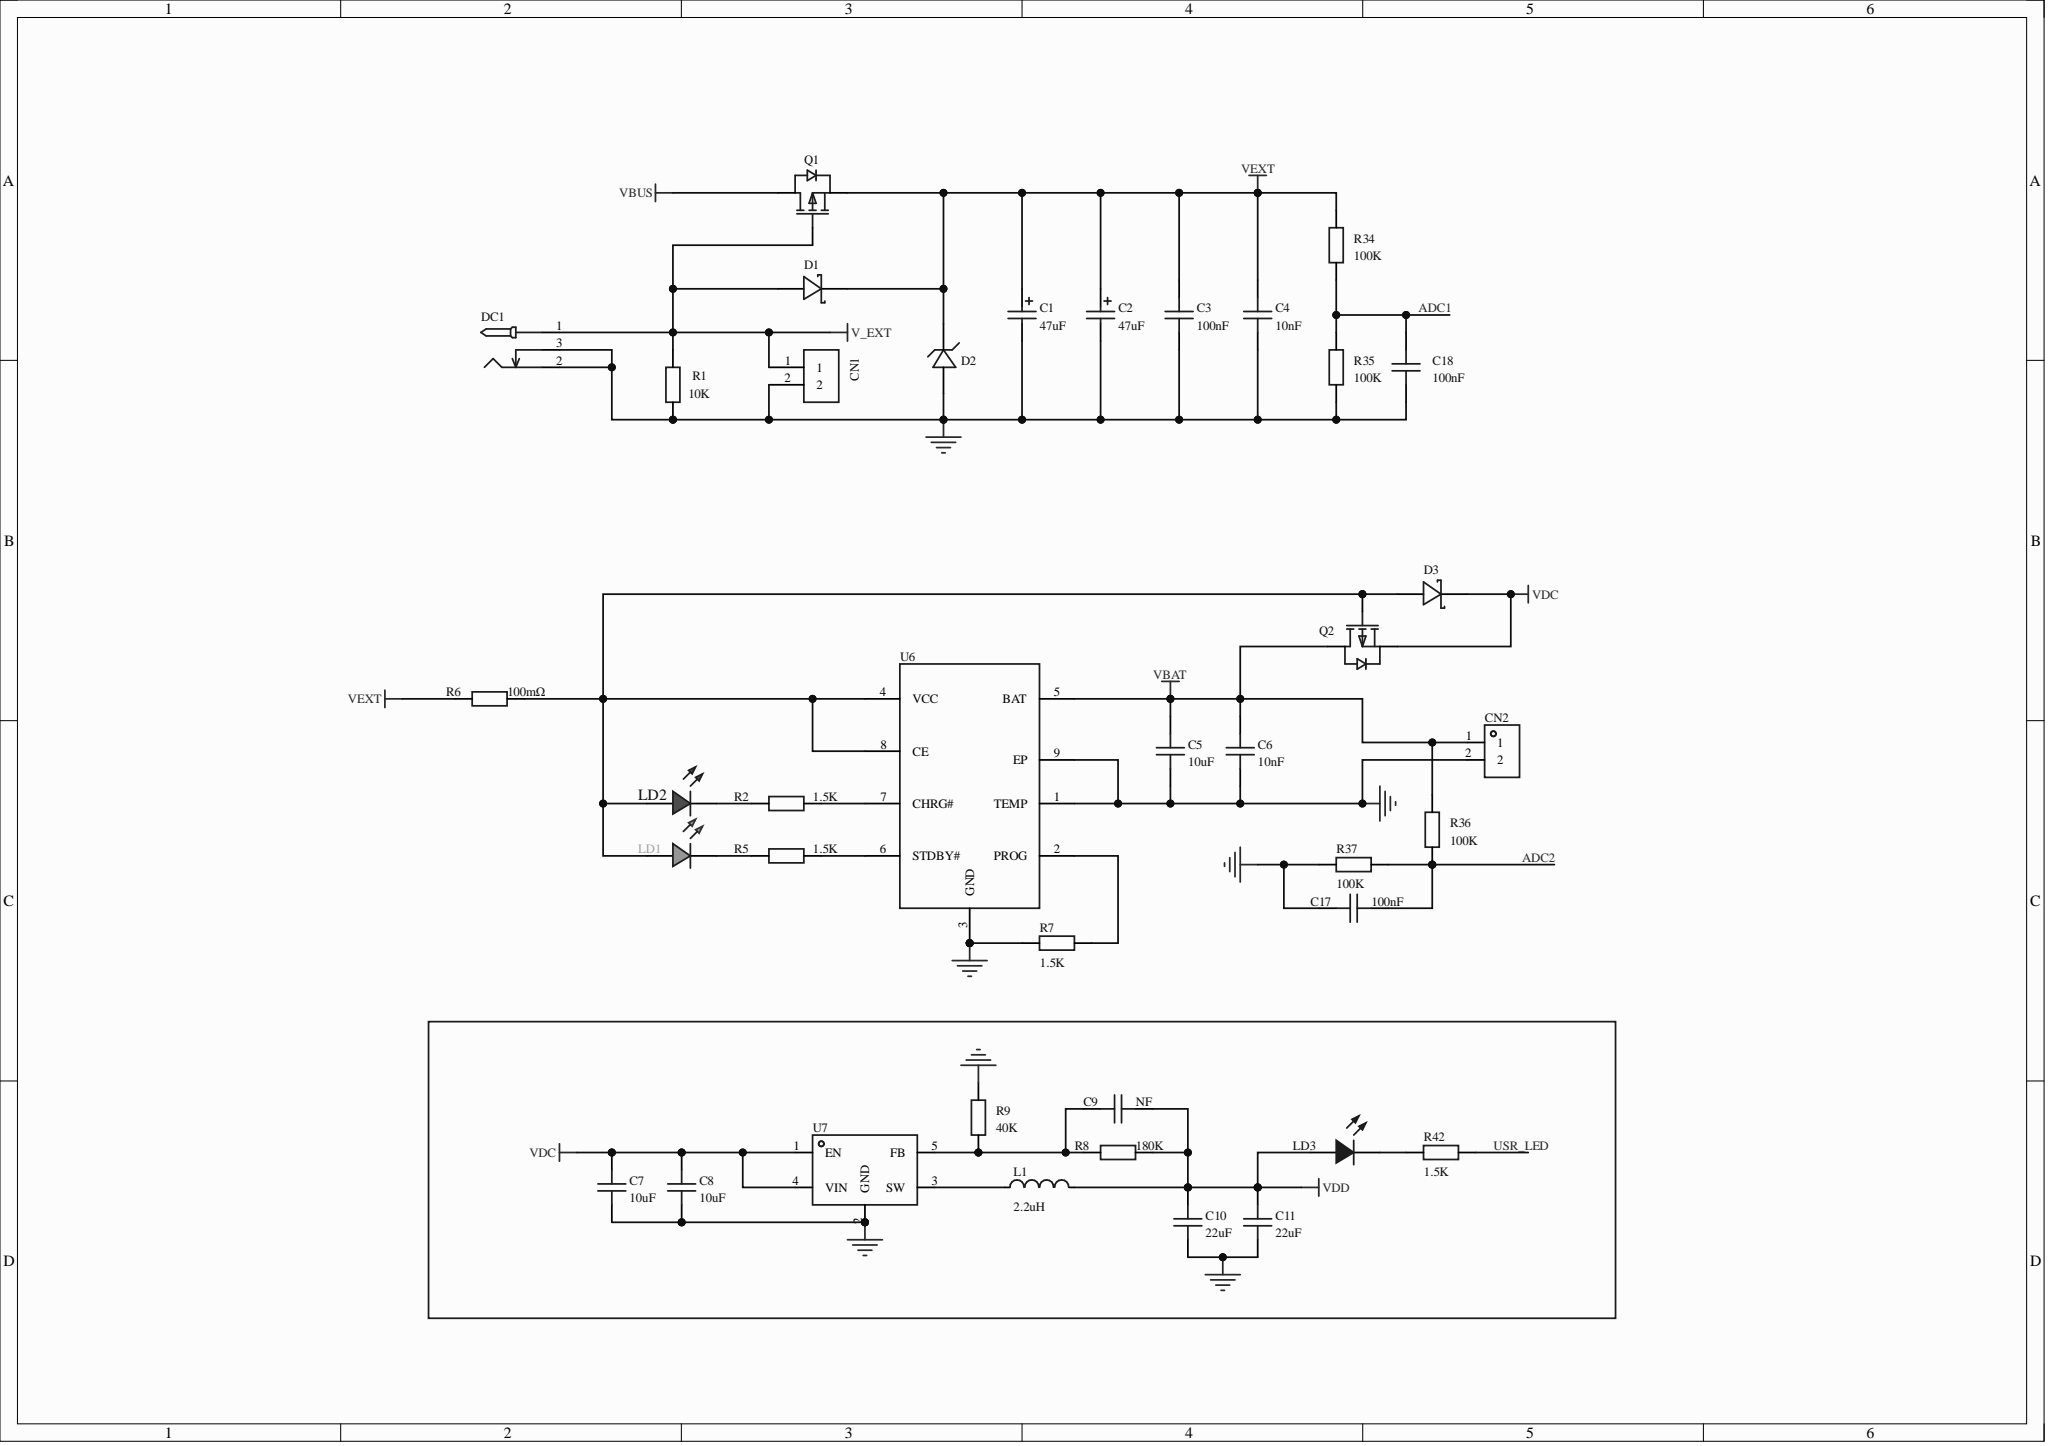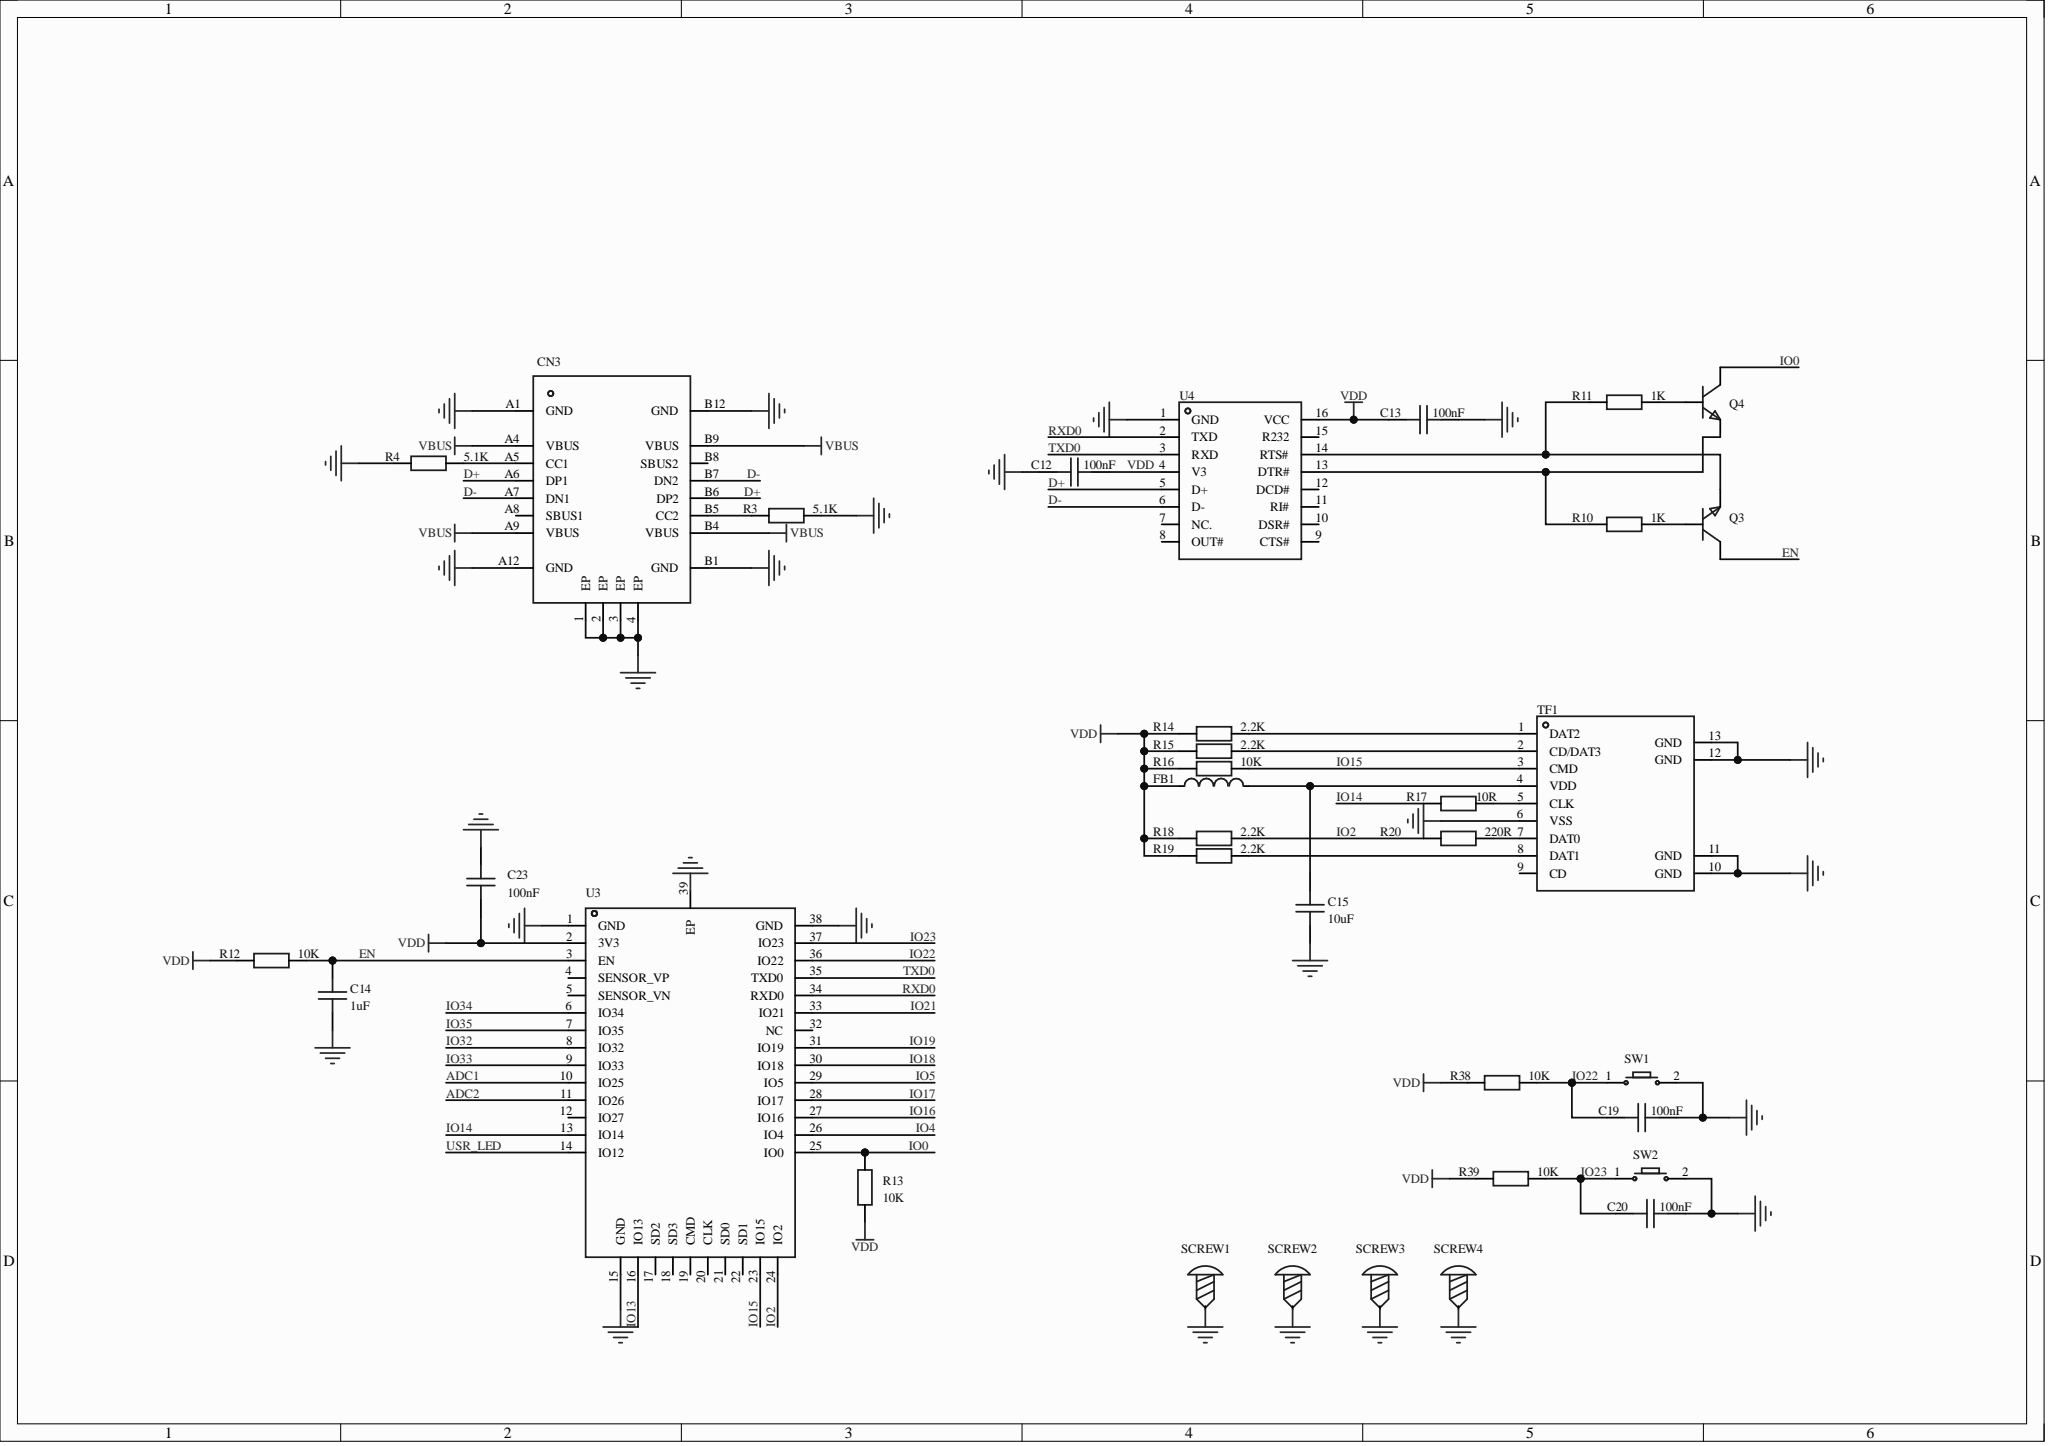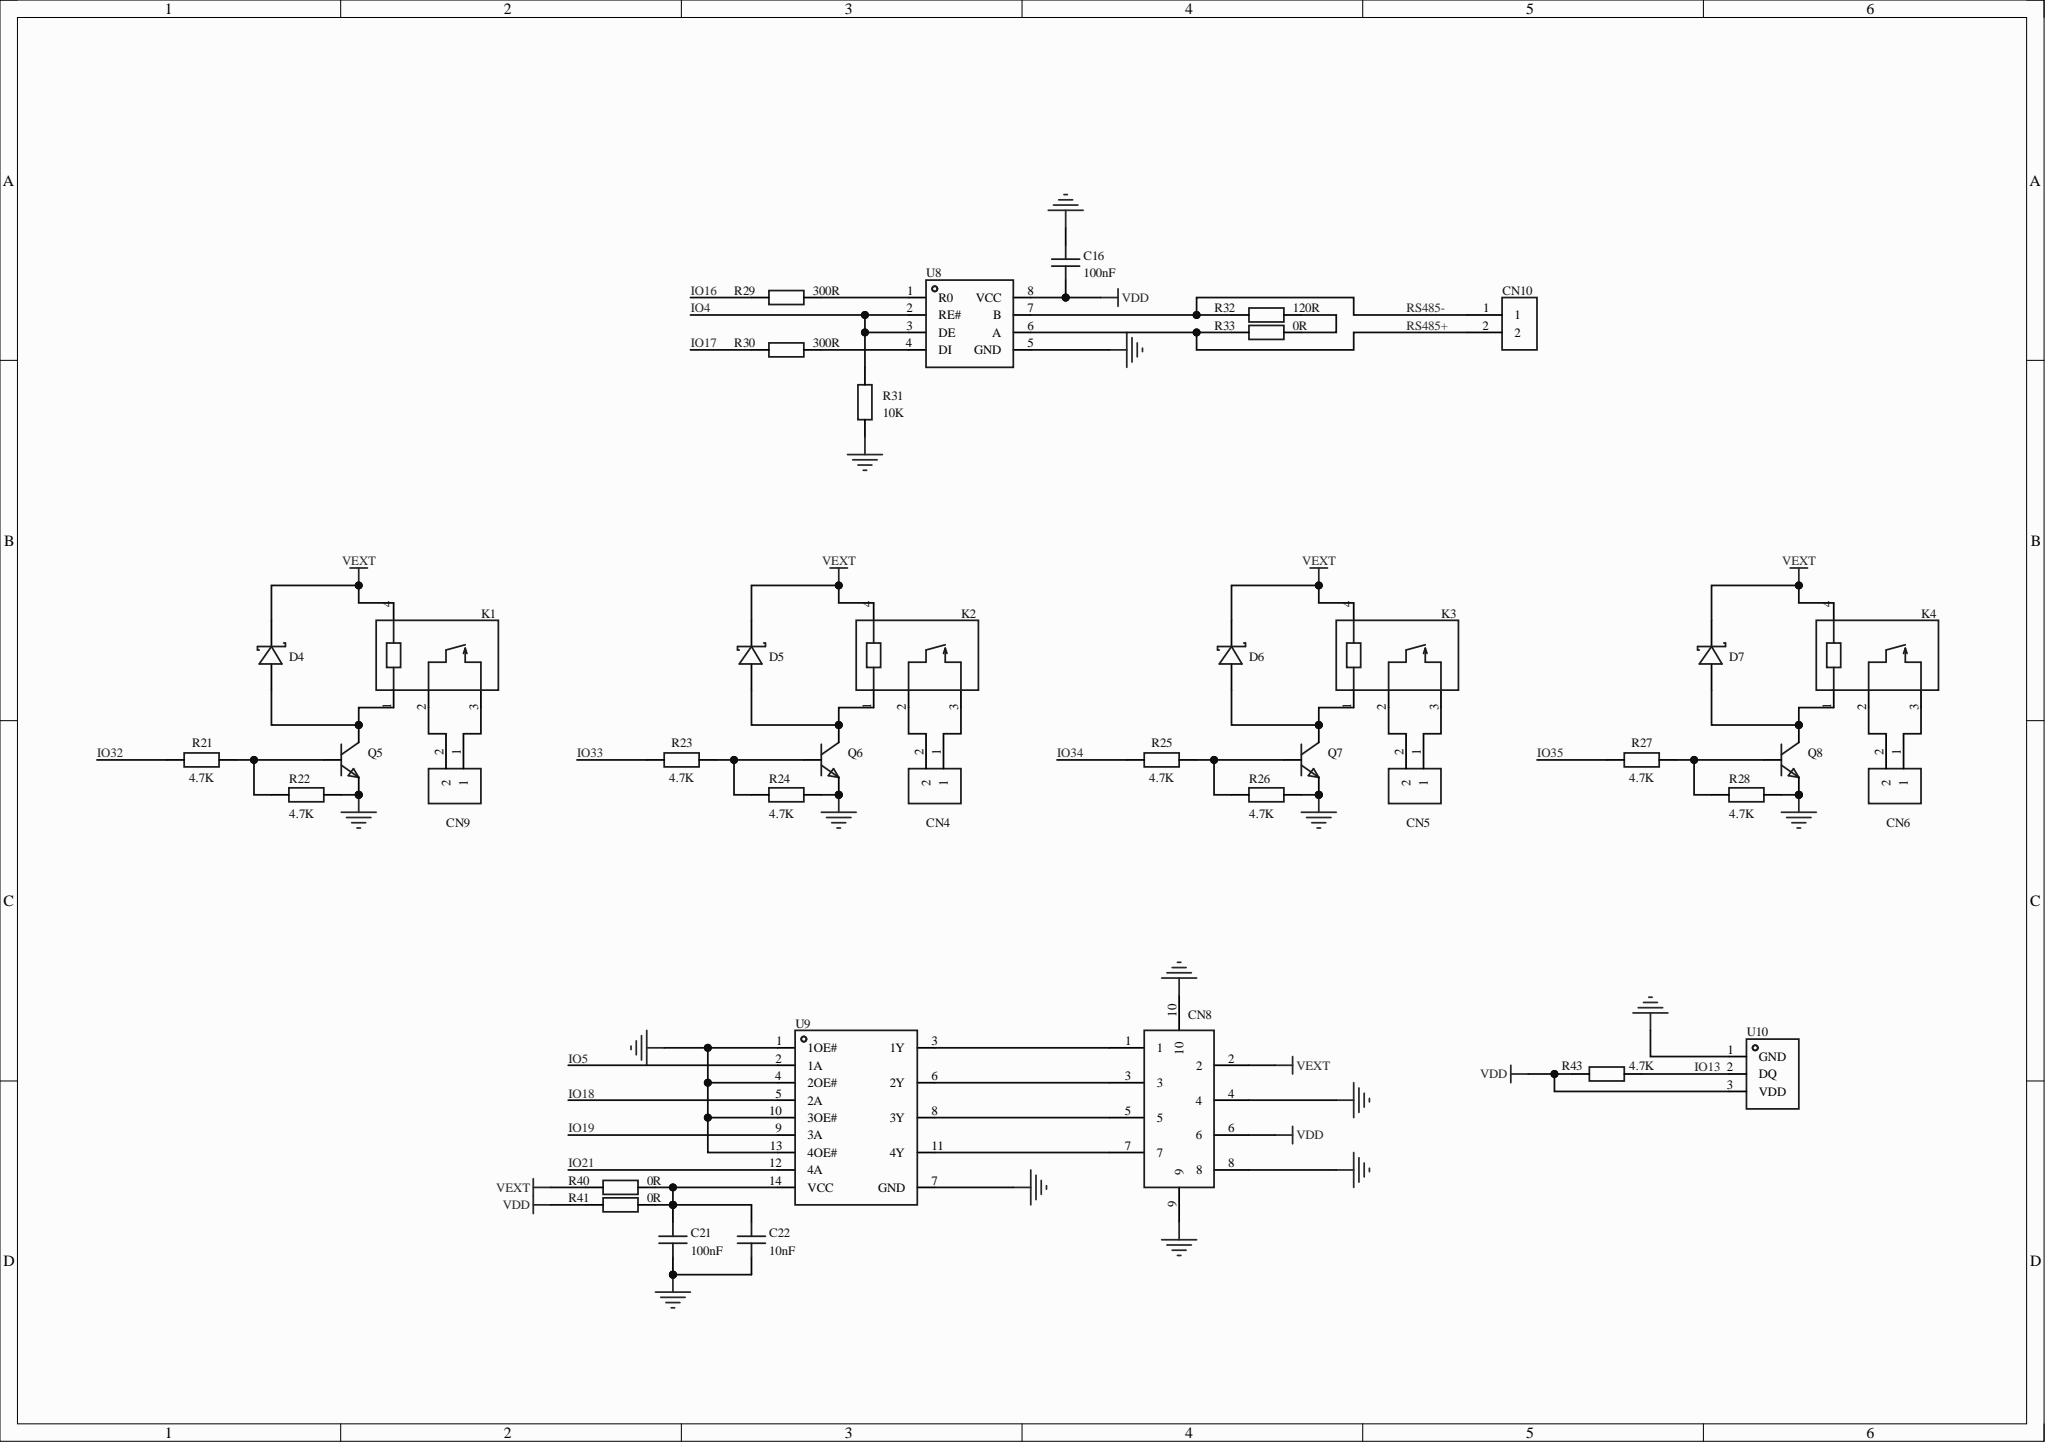Circuit board | Altium Designer | 114 parts | 80 nets
Bill of materials:
Comment,Description,Designator,Footprint,LibRef,Quantity
"C_Ele_SMD_5x5.4mm","","C1, C2","C_Ele_SMD_4x5.5mm","C_Ele_SMD_5x5.4mm","2"
"CAP_0805","","C3, C4, C5, C6, C7, C8, C9, C10, C11, C12, C13, C14, C15, C16, C17, C18, C19, C20, C21, C22, C23","C0805","CAP_0805","21"
"WJ500V-5.08-2P","","CN1, CN4, CN5, CN6, CN9, CN10","CONN-TH_2P-P5.00_WJ500V-5.08-2P","WJ500V-5.08-2P","6"
"ZX-XH2.54-2PZZ","","CN2","CONN-TH_2P-P2.50_HX25003-2A","ZX-XH2.54-2PZZ","1"
"USB_TYPE-C-16P","","CN3","USB_TYPE-C-16P","USB_TYPE-C-16P","1"
"8P-SMD with latch","","CN8","FPC-SMD_8P-P0.50_AFC11-S08ICC-00","8P-立贴带锁","1"
"SS34_C154551","","D1, D3, D4, D5, D6, D7","SMC_L6.9-W5.9-LS7.9-RD","SS34_C154551","6"
"SMBJ6.0A_C2987966","","D2","SMB_L4.6-W3.6-LS5.3-RD","SMBJ6.0A_C2987966","1"
"DC-005_2.5","","DC1","DC-005_2.5","DC-005_2.5","1"
"L_0805","","FB1","L0805","L_0805","1"
"G5NB-1A-E-12VDC","","K1, K2, K3, K4","RELAY-TH_G5NB-1A-E-DCXX","G5NB-1A-E-12VDC","4"
"FXL0420-2R2-M","","L1","IND-SMD_L4.4-W4.2","FXL0420-2R2-M","1"
"LED_0805-G","","LD1","LED_0805","LED_0805-G","1"
"LED_0805-R","","LD2","LED_0805","LED_0805-R","1"
"LED_0805-B","","LD3","LED_0805","LED_0805-B","1"
"AO3401A_C15127","","Q1, Q2","SOT-23_L2.9-W1.3-P1.90-LS2.4-BR","AO3401A_C15127","2"
"SS8050_C7420370","","Q3, Q4, Q5, Q6, Q7, Q8","SOT-23-3_L2.9-W1.3-P1.90-LS2.4-BR","SS8050_C7420370","6"
"Res_0805","","R1, R2, R3, R4, R5, R7, R8, R9, R10, R11, R12, R13, R14, R15, R16, R17, R18, R19, R20, R21, R22, R23, R24, R25, R26, R27, R28, R29, R30, R31, R32, R33, R34, R35, R36, R37, R38, R39, R40, R41, R42, R43","R0805","Res_0805","42"
"1210W2F100LT5E","","R6","R1210","1210W2F100LT5E","1"
"M2 screw","","SCREW1, SCREW2, SCREW3, SCREW4","M2螺丝","M2螺丝","4"
"Key_SMD_3x4x2","","SW1, SW2","Key_SMD_3x4x2","Key_SMD_3x4x2","2"
"TF-CARD H1.8","","TF1","TF-SMD_TF-CARD-H1.8","TF-CARD H1.8","1"
"ESP32-WROOM-32","","U3","WIFIM-SMD_ESP-WROOM-32","ESP32-WROOM-32","1"
"CH340C","","U4","SOP-16_L10.0-W3.9-P1.27-LS6.0-BL","CH340C","1"
"TP4056-42-ESOP8","","U6","ESOP-8_L4.9-W3.9-P1.27-LS6.0-BL-EP","TP4056-42-ESOP8","1"
"","","U7","SOT_XDC","XDC","1"
"MAX485EIM/TR","","U8","SOP-8_L4.9-W3.9-P1.27-LS6.0-BL","MAX485EIM/TR","1"
"74HC125D/S400118","","U9","SOIC-14_L8.6-W3.8-P1.27-LS6.0-BL","74HC125D/S400118","1"
"","","U10","TO-92-3_L4.9-W3.7-P1.27-L","GX18B20","1"
Netlist (Protel format):
[
C1
C_Ele_SMD_4x5.5mm
C_Ele_SMD_5x5.4mm



]
[
C2
C_Ele_SMD_4x5.5mm
C_Ele_SMD_5x5.4mm



]
[
C3
C0805
CAP_0805



]
[
C4
C0805
CAP_0805



]
[
C5
C0805
CAP_0805



]
[
C6
C0805
CAP_0805



]
[
C7
C0805
CAP_0805



]
[
C8
C0805
CAP_0805



]
[
C9
C0805
CAP_0805



]
[
C10
C0805
CAP_0805



]
[
C11
C0805
CAP_0805



]
[
C12
C0805
CAP_0805



]
[
C13
C0805
CAP_0805



]
[
C14
C0805
CAP_0805



]
[
C15
C0805
CAP_0805



]
[
C16
C0805
CAP_0805



]
[
C17
C0805
CAP_0805



]
[
C18
C0805
CAP_0805



]
[
C19
C0805
CAP_0805



]
[
C20
C0805
CAP_0805



]
[
C21
C0805
CAP_0805



]
[
C22
C0805
CAP_0805



]
[
C23
C0805
CAP_0805



]
[
CN1
CONN-TH_2P-P5.00_WJ500V-5.08-2P
WJ500V-5.08-2P



]
[
CN2
CONN-TH_2P-P2.50_HX25003-2A
ZX-XH2.54-2PZZ



]
[
CN3
USB_TYPE-C-16P
USB_TYPE-C-16P



]
[
CN4
CONN-TH_2P-P5.00_WJ500V-5.08-2P
WJ500V-5.08-2P



]
[
CN5
CONN-TH_2P-P5.00_WJ500V-5.08-2P
WJ500V-5.08-2P



]
[
CN6
CONN-TH_2P-P5.00_WJ500V-5.08-2P
WJ500V-5.08-2P



]
[
CN8
FPC-SMD_8P-P0.50_AFC11-S08ICC-00
8P-SMD with latch



]
[
CN9
CONN-TH_2P-P5.00_WJ500V-5.08-2P
WJ500V-5.08-2P



]
[
CN10
CONN-TH_2P-P5.00_WJ500V-5.08-2P
WJ500V-5.08-2P



]
[
D1
SMC_L6.9-W5.9-LS7.9-RD
SS34_C154551



]
[
D2
SMB_L4.6-W3.6-LS5.3-RD
SMBJ6.0A_C2987966



]
[
D3
SMC_L6.9-W5.9-LS7.9-RD
SS34_C154551



]
[
D4
SMC_L6.9-W5.9-LS7.9-RD
SS34_C154551



]
[
D5
SMC_L6.9-W5.9-LS7.9-RD
SS34_C154551



]
[
D6
SMC_L6.9-W5.9-LS7.9-RD
SS34_C154551



]
[
D7
SMC_L6.9-W5.9-LS7.9-RD
SS34_C154551



]
[
DC1
DC-005_2.5
DC-005_2.5



]
[
FB1
L0805
L_0805



]
[
K1
RELAY-TH_G5NB-1A-E-DCXX
G5NB-1A-E-12VDC



]
[
K2
RELAY-TH_G5NB-1A-E-DCXX
G5NB-1A-E-12VDC



]
[
K3
RELAY-TH_G5NB-1A-E-DCXX
G5NB-1A-E-12VDC



]
[
K4
RELAY-TH_G5NB-1A-E-DCXX
G5NB-1A-E-12VDC



]
[
L1
IND-SMD_L4.4-W4.2
FXL0420-2R2-M



]
[
LD1
LED_0805
LED_0805-G



]
[
LD2
LED_0805
LED_0805-R



]
[
LD3
LED_0805
LED_0805-B



]
[
Q1
SOT-23_L2.9-W1.3-P1.90-LS2.4-BR
AO3401A_C15127



]
[
Q2
SOT-23_L2.9-W1.3-P1.90-LS2.4-BR
AO3401A_C15127



]
[
Q3
SOT-23-3_L2.9-W1.3-P1.90-LS2.4-BR
SS8050_C7420370



]
[
Q4
SOT-23-3_L2.9-W1.3-P1.90-LS2.4-BR
SS8050_C7420370



]
[
Q5
SOT-23-3_L2.9-W1.3-P1.90-LS2.4-BR
SS8050_C7420370



]
[
Q6
SOT-23-3_L2.9-W1.3-P1.90-LS2.4-BR
SS8050_C7420370



]
[
Q7
SOT-23-3_L2.9-W1.3-P1.90-LS2.4-BR
SS8050_C7420370



]
[
Q8
SOT-23-3_L2.9-W1.3-P1.90-LS2.4-BR
SS8050_C7420370



]
[
R1
R0805
Res_0805



]
[
R2
R0805
Res_0805



]
[
R3
R0805
Res_0805



]
[
R4
R0805
Res_0805



]
[
R5
R0805
Res_0805



]
[
R6
R1210
1210W2F100LT5E



]
[
R7
R0805
Res_0805



]
[
R8
R0805
Res_0805



]
[
R9
R0805
Res_0805



]
[
R10
R0805
Res_0805



]
[
R11
R0805
Res_0805



]
[
R12
R0805
Res_0805



]
[
R13
R0805
Res_0805



]
[
R14
R0805
Res_0805



]
[
R15
R0805
Res_0805



]
[
R16
R0805
Res_0805



]
[
R17
R0805
Res_0805



]
[
R18
R0805
Res_0805



]
[
R19
R0805
Res_0805



]
[
R20
R0805
Res_0805



]
[
R21
R0805
Res_0805



]
[
R22
R0805
Res_0805



]
[
R23
R0805
Res_0805



]
[
R24
R0805
Res_0805



]
[
R25
R0805
Res_0805



]
[
R26
R0805
Res_0805



]
[
R27
R0805
Res_0805



]
[
R28
R0805
Res_0805



]
[
R29
R0805
Res_0805



]
[
R30
R0805
Res_0805



]
[
R31
R0805
Res_0805



]
[
R32
R0805
Res_0805



]
[
R33
R0805
Res_0805



]
[
R34
R0805
Res_0805



]
[
R35
R0805
Res_0805



]
[
R36
R0805
Res_0805



]
[
R37
R0805
Res_0805



]
[
R38
R0805
Res_0805



]
[
R39
R0805
Res_0805



]
[
R40
R0805
Res_0805



]
[
R41
R0805
Res_0805



]
[
R42
R0805
Res_0805



]
[
R43
R0805
Res_0805



]
[
SCREW1
M2螺丝
M2 screw



]
[
SCREW2
M2螺丝
M2 screw



]
[
SCREW3
M2螺丝
M2 screw



]
[
SCREW4
M2螺丝
M2 screw



]
[
SW1
Key_SMD_3x4x2
Key_SMD_3x4x2



]
[
SW2
Key_SMD_3x4x2
Key_SMD_3x4x2



]
[
TF1
TF-SMD_TF-CARD-H1.8
TF-CARD H1.8



]
[
U3
WIFIM-SMD_ESP-WROOM-32
ESP32-WROOM-32



]
[
U4
SOP-16_L10.0-W3.9-P1.27-LS6.0-BL
CH340C



]
[
U6
ESOP-8_L4.9-W3.9-P1.27-LS6.0-BL-EP
TP4056-42-ESOP8



]
[
U7
SOT_XDC




]
[
U8
SOP-8_L4.9-W3.9-P1.27-LS6.0-BL
MAX485EIM/TR



]
[
U9
SOIC-14_L8.6-W3.8-P1.27-LS6.0-BL
74HC125D/S400118



]
[
U10
TO-92-3_L4.9-W3.7-P1.27-L




]
(
VEXT
C1-1
C2-1
C3-2
C4-2
CN8-2
D1-1
D2-1
D4-1
D5-1
D6-1
D7-1
K1-4
K2-4
K3-4
K4-4
Q1-2
R6-1
R34-1
R40-2
)
(
VDD
C9-1
C10-2
C11-2
C12-1
C13-2
C16-1
C23-1
CN8-6
FB1-1
L1-2
LD3-2
R8-2
R12-2
R13-2
R14-2
R15-2
R16-2
R18-2
R19-2
R38-2
R39-2
R41-2
R43-2
U3-2
U4-4
U4-16
U8-8
U10-3
)
(
VDC
C7-2
C8-2
D3-1
Q2-2
U7-1
U7-4
)
(
VBUS
CN3-A4
CN3-A9
CN3-B4
CN3-B9
Q1-3
)
(
VBAT
C5-2
C6-2
CN2-1
Q2-3
R36-2
U6-5
)
(
V_EXT
CN1-1
D1-2
DC1-1
Q1-1
R1-2
)
(
USR_LED
R42-2
U3-14
)
(
TXD0
U3-35
U4-3
)
(
RXD0
U3-34
U4-2
)
(
RS485-
CN10-1
R32-1
U8-7
)
(
RS485+
CN10-2
R33-1
U8-6
)
(
NetR32_2
R32-2
R33-2
)
(
NetR30_1
R30-1
U8-4
)
(
NetR29_1
R29-1
U8-1
)
(
NetR20_1
R20-1
TF1-7
)
(
NetR19_1
R19-1
TF1-8
)
(
NetR17_1
R17-1
TF1-5
)
(
NetR15_1
R15-1
TF1-2
)
(
NetR14_1
R14-1
TF1-1
)
(
NetR7_1
R7-1
U6-2
)
(
NetR5_1
R5-1
U6-6
)
(
NetR2_1
R2-1
U6-7
)
(
NetQ8_1
Q8-1
R27-1
R28-2
)
(
NetQ7_1
Q7-1
R25-1
R26-2
)
(
NetQ6_1
Q6-1
R23-1
R24-2
)
(
NetQ5_1
Q5-1
R21-1
R22-2
)
(
NetQ4_2
Q4-2
R10-2
U4-13
)
(
NetQ4_1
Q4-1
R11-1
)
(
NetQ3_2
Q3-2
R11-2
U4-14
)
(
NetQ3_1
Q3-1
R10-1
)
(
NetLD3_1
LD3-1
R42-1
)
(
NetLD2_1
LD2-1
R2-2
)
(
NetLD1_1
LD1-1
R5-2
)
(
NetL1_1
L1-1
U7-3
)
(
NetD7_2
D7-2
K4-1
Q8-3
)
(
NetD6_2
D6-2
K3-1
Q7-3
)
(
NetD5_2
D5-2
K2-1
Q6-3
)
(
NetD4_2
D4-2
K1-1
Q5-3
)
(
NetD3_2
D3-2
LD1-2
LD2-2
Q2-1
R6-2
U6-4
U6-8
)
(
NetCN9_2
CN9-2
K1-2
)
(
NetCN9_1
CN9-1
K1-3
)
(
NetCN8_7
CN8-7
U9-11
)
(
NetCN8_5
CN8-5
U9-8
)
(
NetCN8_3
CN8-3
U9-6
)
(
NetCN8_1
CN8-1
U9-3
)
(
NetCN6_2
CN6-2
K4-2
)
(
NetCN6_1
CN6-1
K4-3
)
(
NetCN5_2
CN5-2
K3-2
)
(
NetCN5_1
CN5-1
K3-3
)
(
NetCN4_2
CN4-2
K2-2
)
(
NetCN4_1
CN4-1
K2-3
)
(
NetCN3_B5
CN3-B5
R3-2
)
(
NetCN3_A5
CN3-A5
R4-2
)
(
NetC21_2
C21-2
C22-2
R40-1
R41-1
U9-14
)
(
NetC15_1
C15-1
FB1-2
TF1-4
)
(
NetC9_2
C9-2
R8-1
R9-2
U7-5
)
(
IO35
R27-2
U3-7
)
(
IO34
R25-2
U3-6
)
(
IO33
R23-2
U3-9
)
(
IO32
R21-2
U3-8
)
(
IO23
C20-2
R39-1
SW2-1
U3-37
)
(
IO22
C19-2
R38-1
SW1-1
U3-36
)
(
IO21
U3-33
U9-12
)
(
IO19
U3-31
U9-9
)
(
IO18
U3-30
U9-5
)
(
IO17
R30-2
U3-28
)
(
IO16
R29-2
U3-27
)
(
IO15
R16-1
TF1-3
U3-23
)
(
IO14
R17-2
U3-13
)
(
IO13
R43-1
U3-16
U10-2
)
(
IO5
U3-29
U9-2
)
(
IO4
R31-1
U3-26
U8-2
U8-3
)
(
IO2
R18-1
R20-2
U3-24
)
(
IO0
Q4-3
R13-1
U3-25
)
(
GND
C1-2
C2-2
C3-1
C4-1
C5-1
C6-1
C7-1
C8-1
C10-1
C11-1
C12-2
C13-1
C14-2
C15-2
C16-2
C17-2
C18-2
C19-1
C20-1
C21-1
C22-1
C23-2
CN1-2
CN2-2
CN3-1
CN3-2
CN3-3
CN3-4
CN3-A1
CN3-A12
CN3-B1
CN3-B12
CN8-4
CN8-8
CN8-9
CN8-10
D2-2
DC1-2
DC1-3
Q5-2
Q6-2
Q7-2
Q8-2
R1-1
R3-1
R4-1
R7-2
R9-1
R22-1
R24-1
R26-1
R28-1
R31-2
R35-2
R37-1
SCREW1-1
SCREW2-1
SCREW3-1
SCREW4-1
SW1-2
SW2-2
TF1-6
TF1-10
TF1-11
TF1-12
TF1-13
U3-1
U3-15
U3-38
U3-39
U4-1
U6-1
U6-3
U6-9
U7-2
U8-5
U9-1
U9-4
U9-7
U9-10
U9-13
U10-1
)
(
EN
C14-1
Q3-3
R12-1
U3-3
)
(
D-
CN3-A7
CN3-B7
U4-6
)
(
D+
CN3-A6
CN3-B6
U4-5
)
(
ADC2
C17-1
R36-1
R37-2
U3-11
)
(
ADC1
C18-1
R34-2
R35-1
U3-10
)